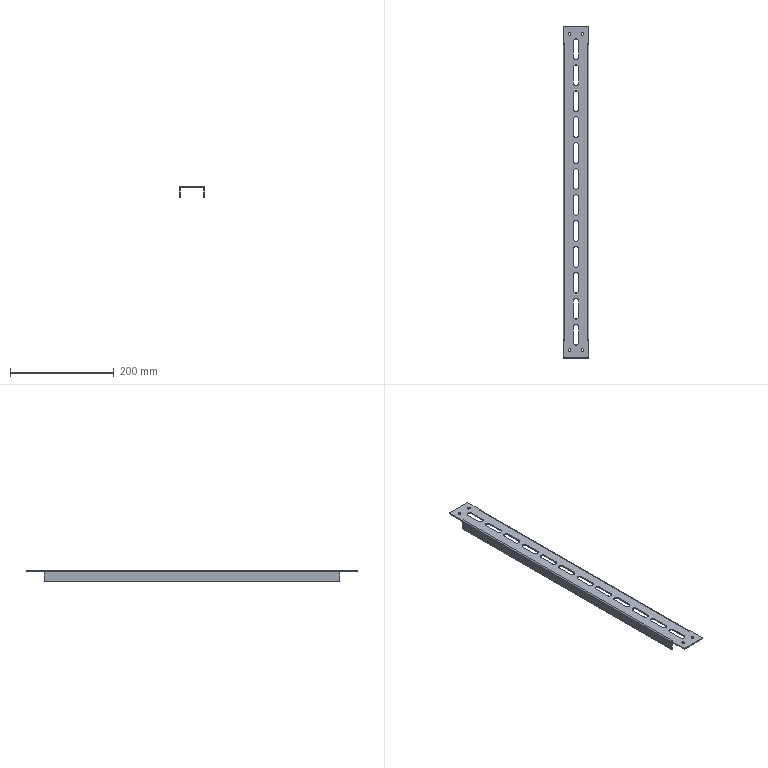Part | STEP file | Transformer bracket | 1 solid | 94 faces | box 50 x 640 x 20 mm | volume 94677 mm3 | plane 58 | cylinder 36 | commonest cylinder face diameters 10 x24 5.3 x8 0.2 x2 4.2 x2